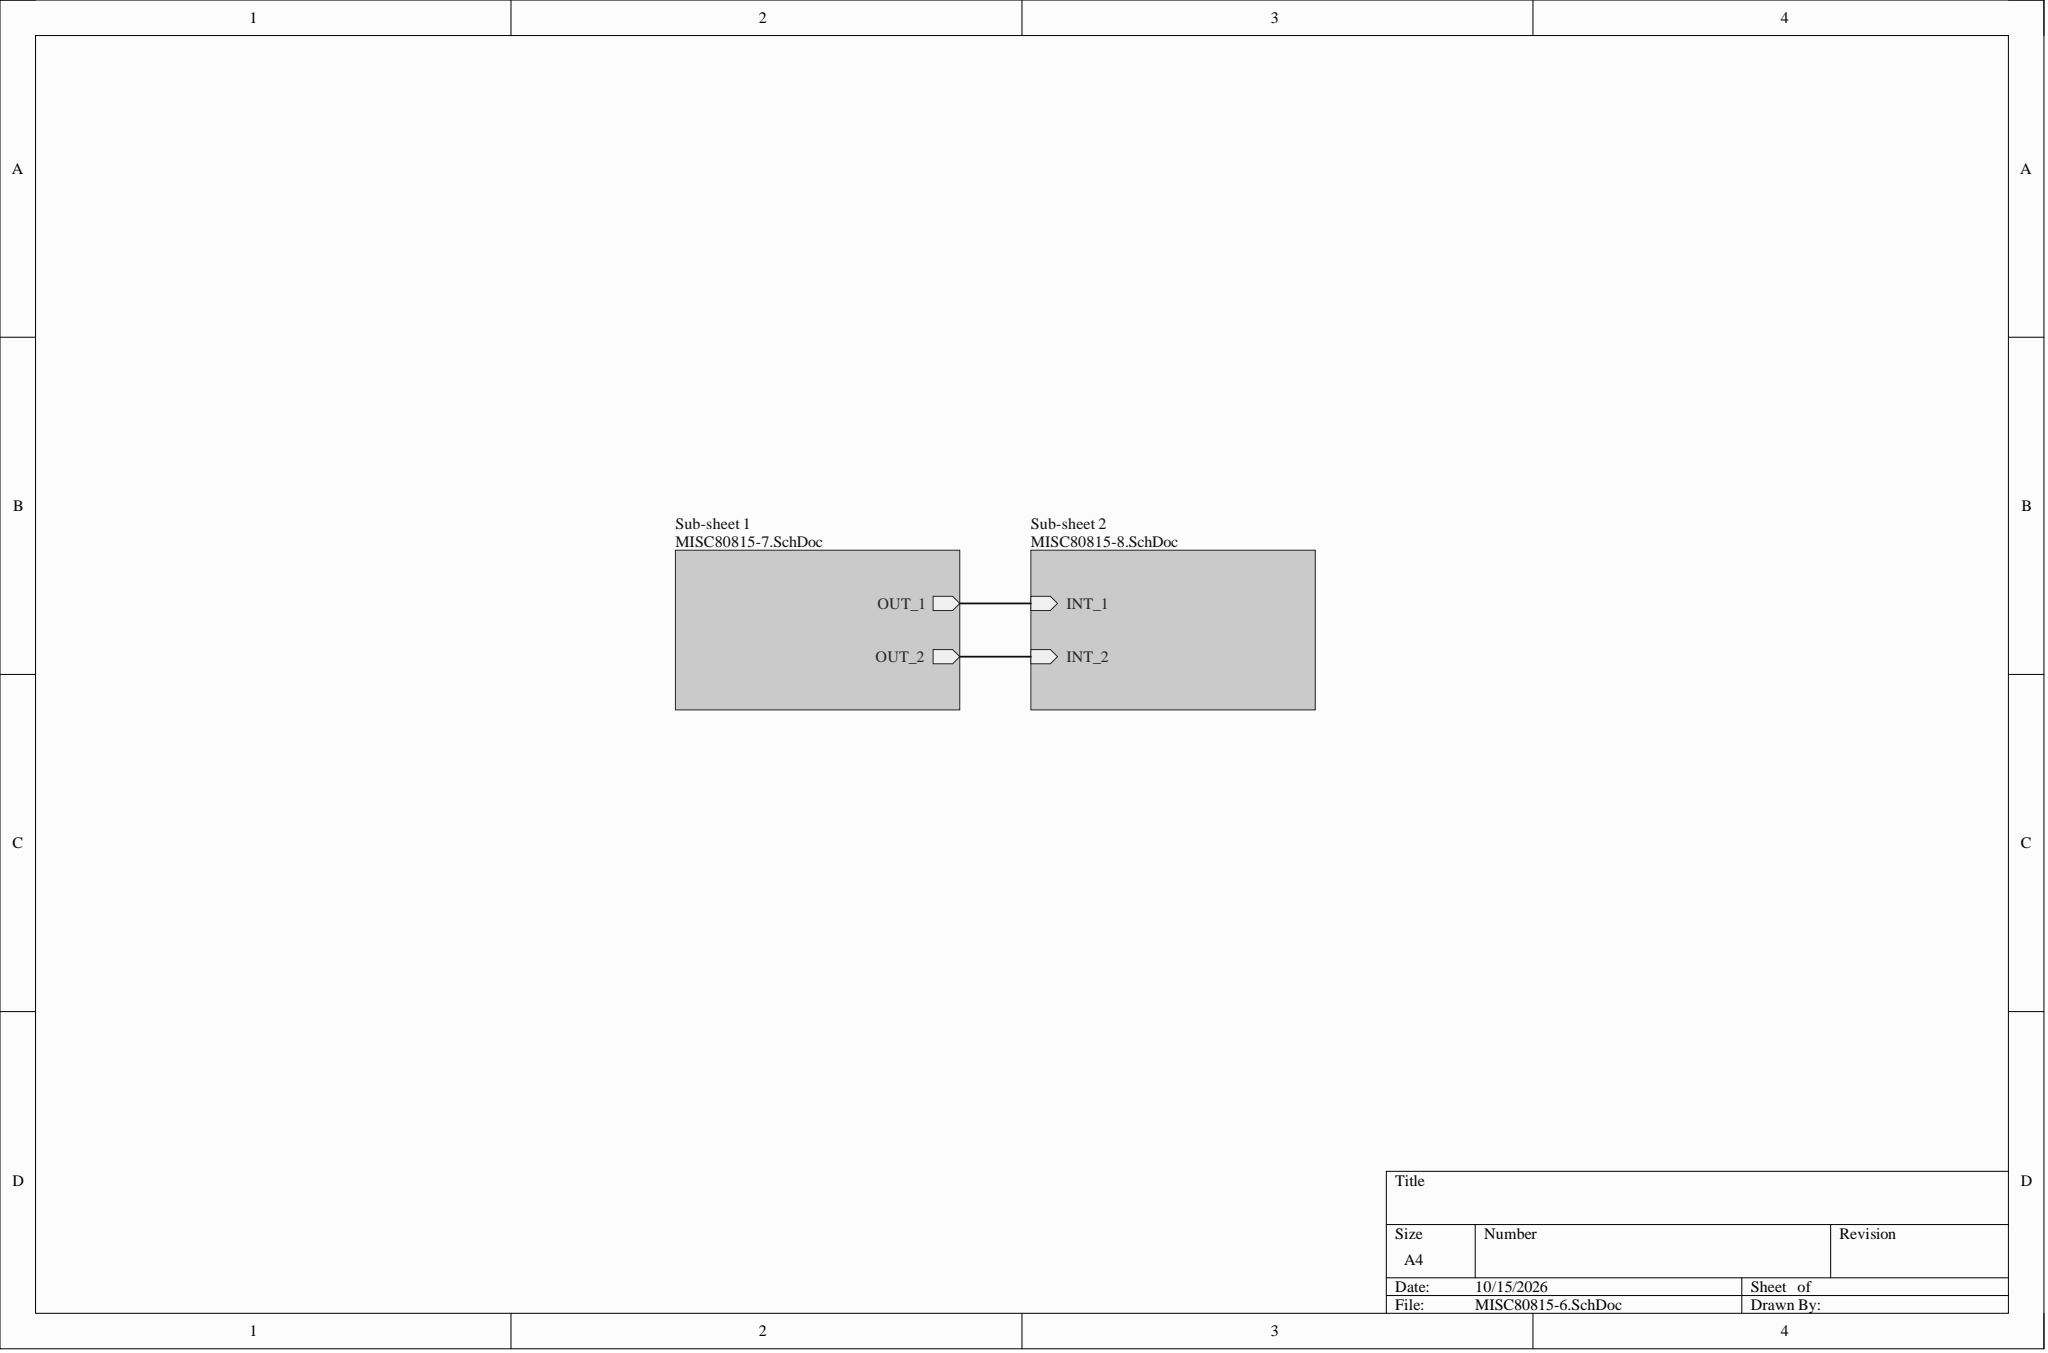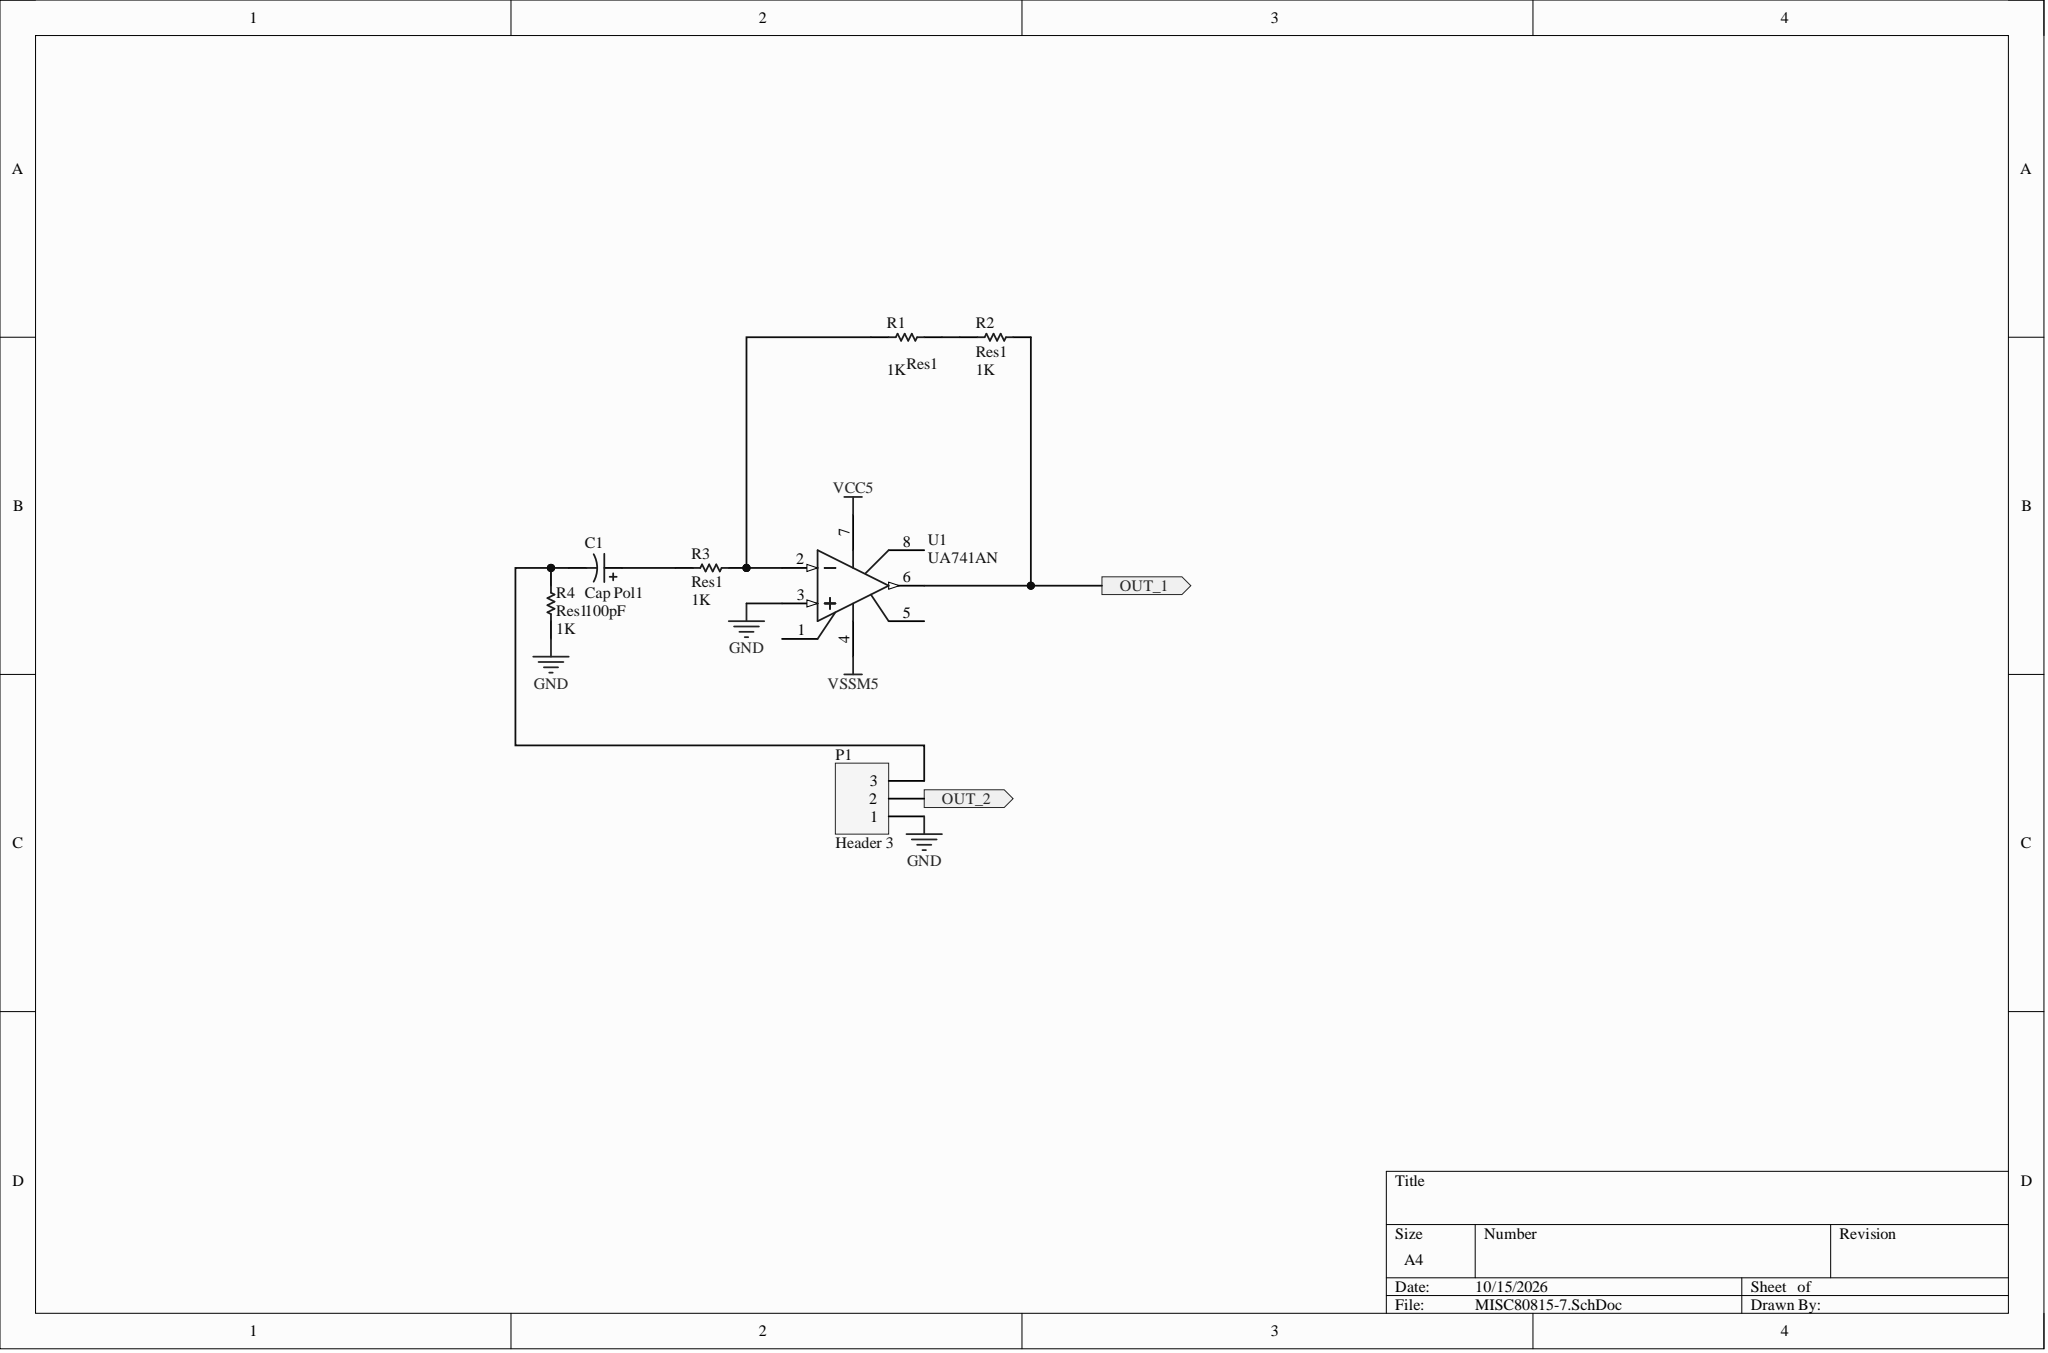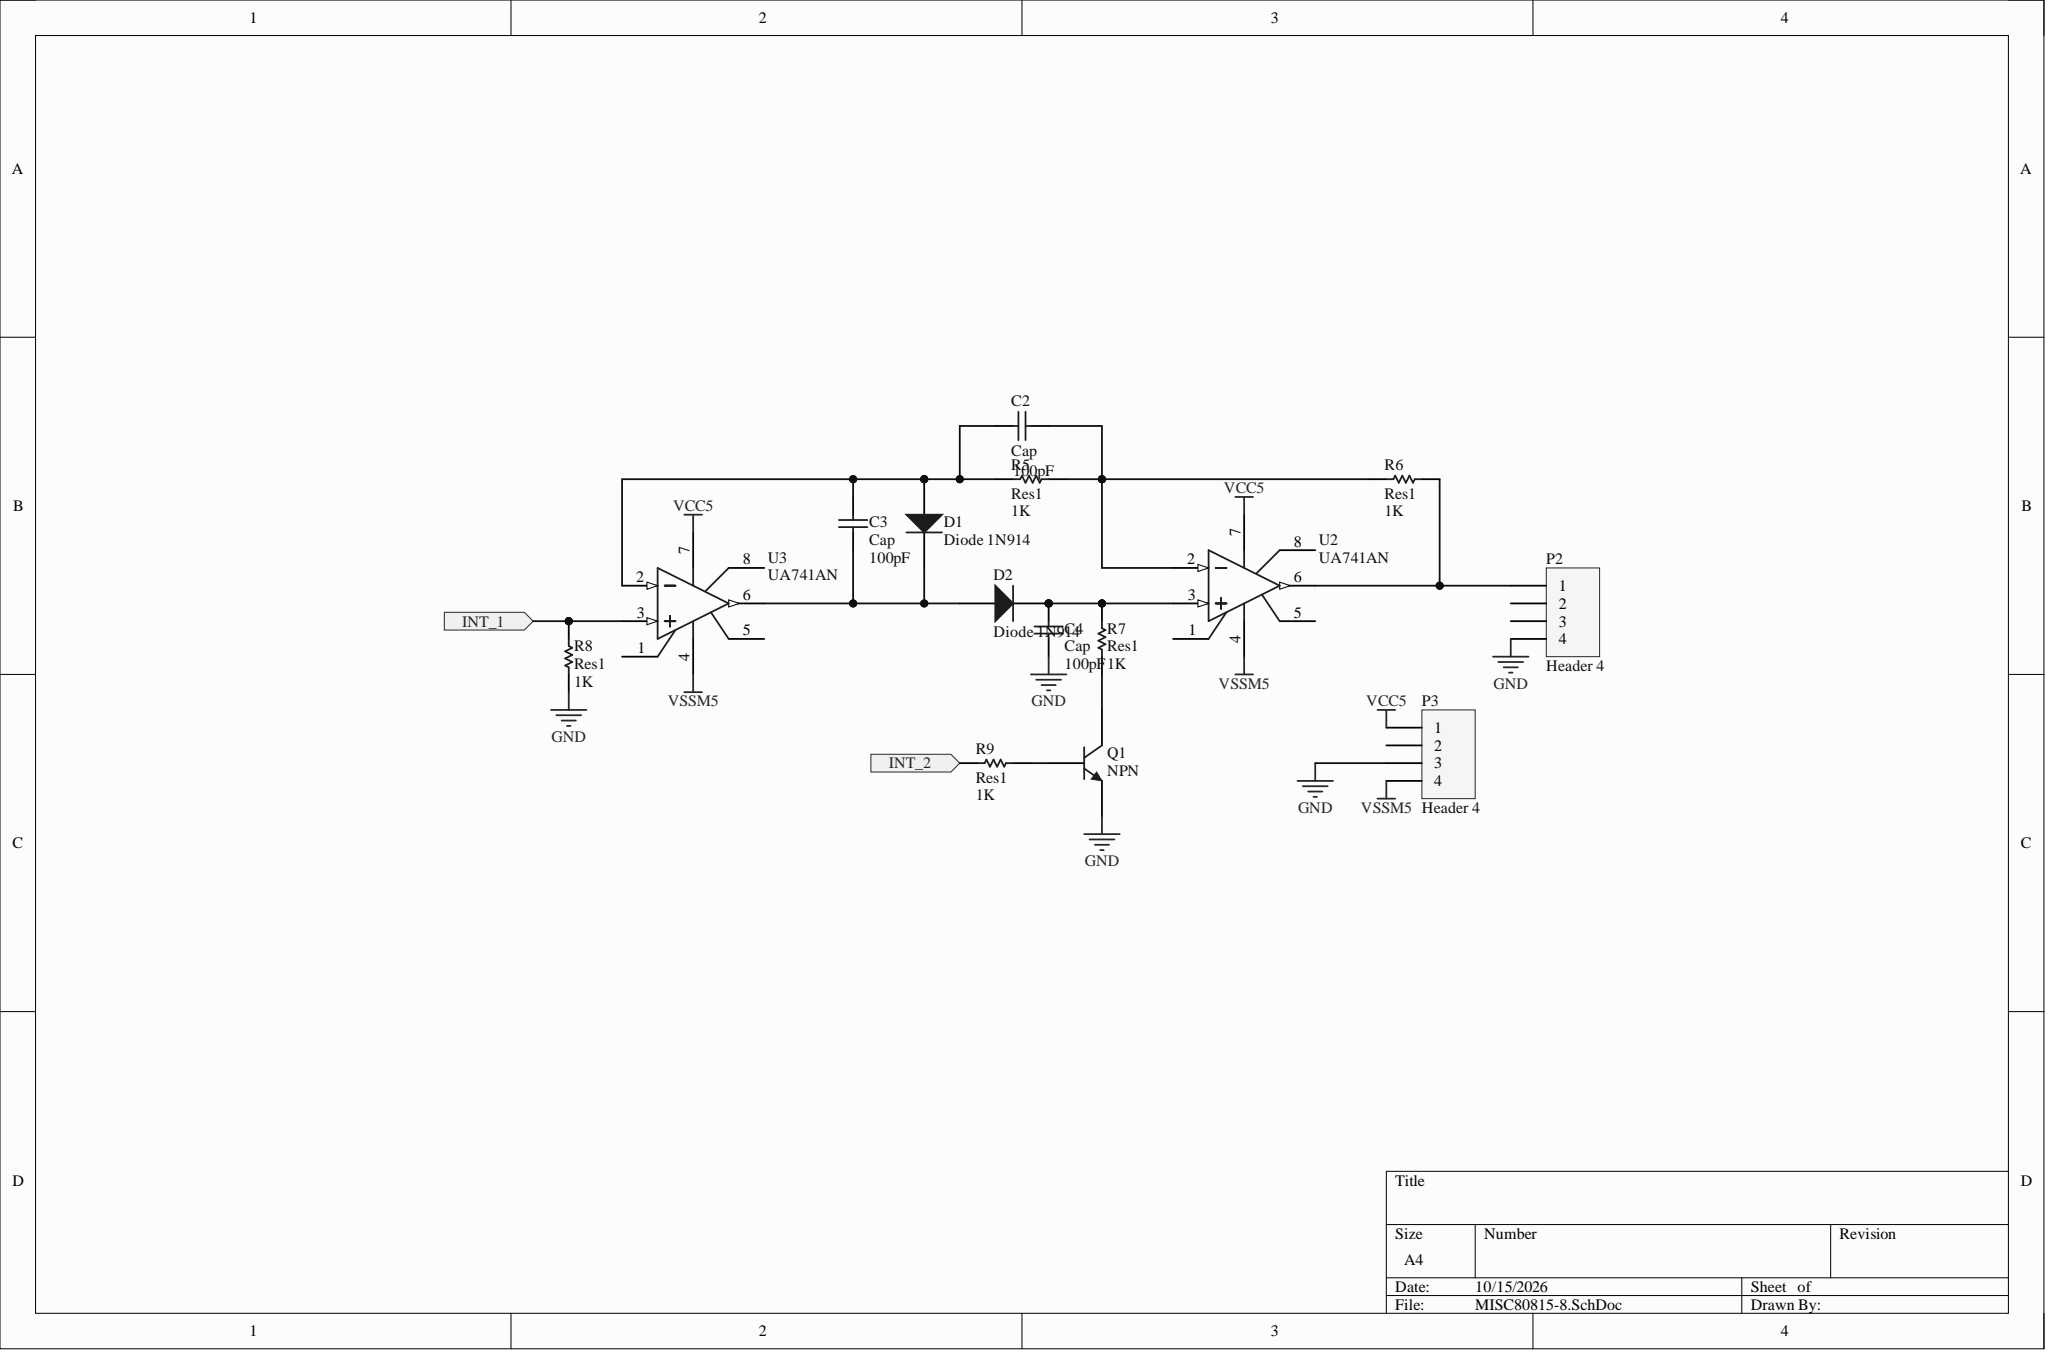Circuit board | Altium Designer | 22 parts | 16 nets
Bill of materials:
Comment,Description,Designator,Footprint,LibRef,Quantity
"Cap Pol1","Polarized Capacitor (Radial)","C1","RB7.6-15","Cap Pol1","1"
"Cap","Capacitor","C2, C3, C4","RAD-0.3","Cap","3"
"Diode 1N914","High Conductance Fast Diode","D1, D2","DO-35","Diode 1N914","2"
"Header 3","Header, 3-Pin","P1","HDR1X3","Header 3","1"
"Header 4","Header, 4-Pin","P2, P3","HDR1X4","Header 4","2"
"NPN","NPN Bipolar Transistor","Q1","TO-226-AA","NPN","1"
"Res1","Resistor","R1, R2, R3, R4, R5, R6, R7, R8, R9","AXIAL-0.3","Res1","9"
"UA741AN","General-Purpose Single Operational Amplifier","U1, U2, U3","DIP-8","UA741AN","3"
Netlist (Protel format):
[
C1
RB7.6-15
Cap Pol1



]
[
C2
RAD-0.3
Cap



]
[
C3
RAD-0.3
Cap



]
[
C4
RAD-0.3
Cap



]
[
D1
DO-35
Diode 1N914



]
[
D2
DO-35
Diode 1N914



]
[
P1
HDR1X3
Header 3



]
[
P2
HDR1X4
Header 4



]
[
P3
HDR1X4
Header 4



]
[
Q1
TO-226-AA
NPN



]
[
R1
AXIAL-0.3
Res1



]
[
R2
AXIAL-0.3
Res1



]
[
R3
AXIAL-0.3
Res1



]
[
R4
AXIAL-0.3
Res1



]
[
R5
AXIAL-0.3
Res1



]
[
R6
AXIAL-0.3
Res1



]
[
R7
AXIAL-0.3
Res1



]
[
R8
AXIAL-0.3
Res1



]
[
R9
AXIAL-0.3
Res1



]
[
U1
DIP-8
UA741AN



]
[
U2
DIP-8
UA741AN



]
[
U3
DIP-8
UA741AN



]
(
VSSM5
P3-4
U1-4
U2-4
U3-4
)
(
VCC5
P3-1
U1-7
U2-7
U3-7
)
(
NetR2_2
R2-2
R8-2
U1-6
U3-3
)
(
NetR1_2
R1-2
R2-1
)
(
NetR1_1
R1-1
R3-2
U1-2
)
(
NetQ1_2
Q1-2
R9-1
)
(
NetQ1_1
Q1-1
R7-2
)
(
NetP2_1
P2-1
R6-2
U2-6
)
(
NetP1_2
P1-2
R9-2
)
(
NetC4_1
C4-1
D2-2
R7-1
U2-3
)
(
NetC3_1
C3-1
D1-2
D2-1
U3-6
)
(
NetC2_2
C2-2
C3-2
D1-1
R5-1
U3-2
)
(
NetC2_1
C2-1
R5-2
R6-1
U2-2
)
(
NetC1_2
C1-2
P1-3
R4-2
)
(
NetC1_1
C1-1
R3-1
)
(
GND
C4-2
P1-1
P2-4
P3-3
Q1-3
R4-1
R8-1
U1-3
)